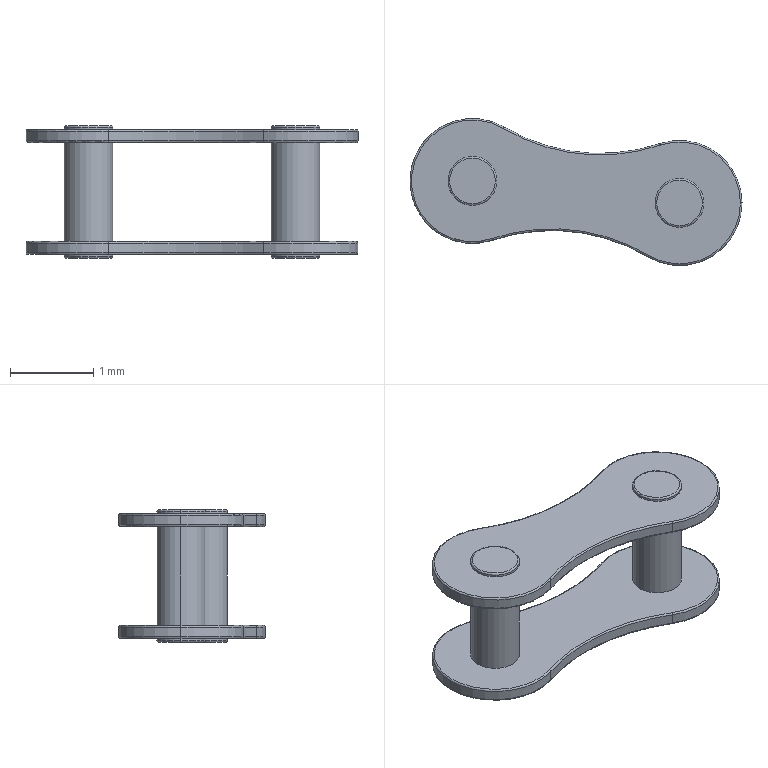Part | SolidWorks | features Scale 3, Extrusion 1, Fillet 1, ICE 1, MirrorSolid 1 | 1 solid | 58 faces | box 3.986 x 1.764 x 1.587 mm | volume 2.162 mm3 | torus 28 | cylinder 22 | plane 8 | commonest cylinder face diameters 0.587 x12 1.5 x6 4.5 x4